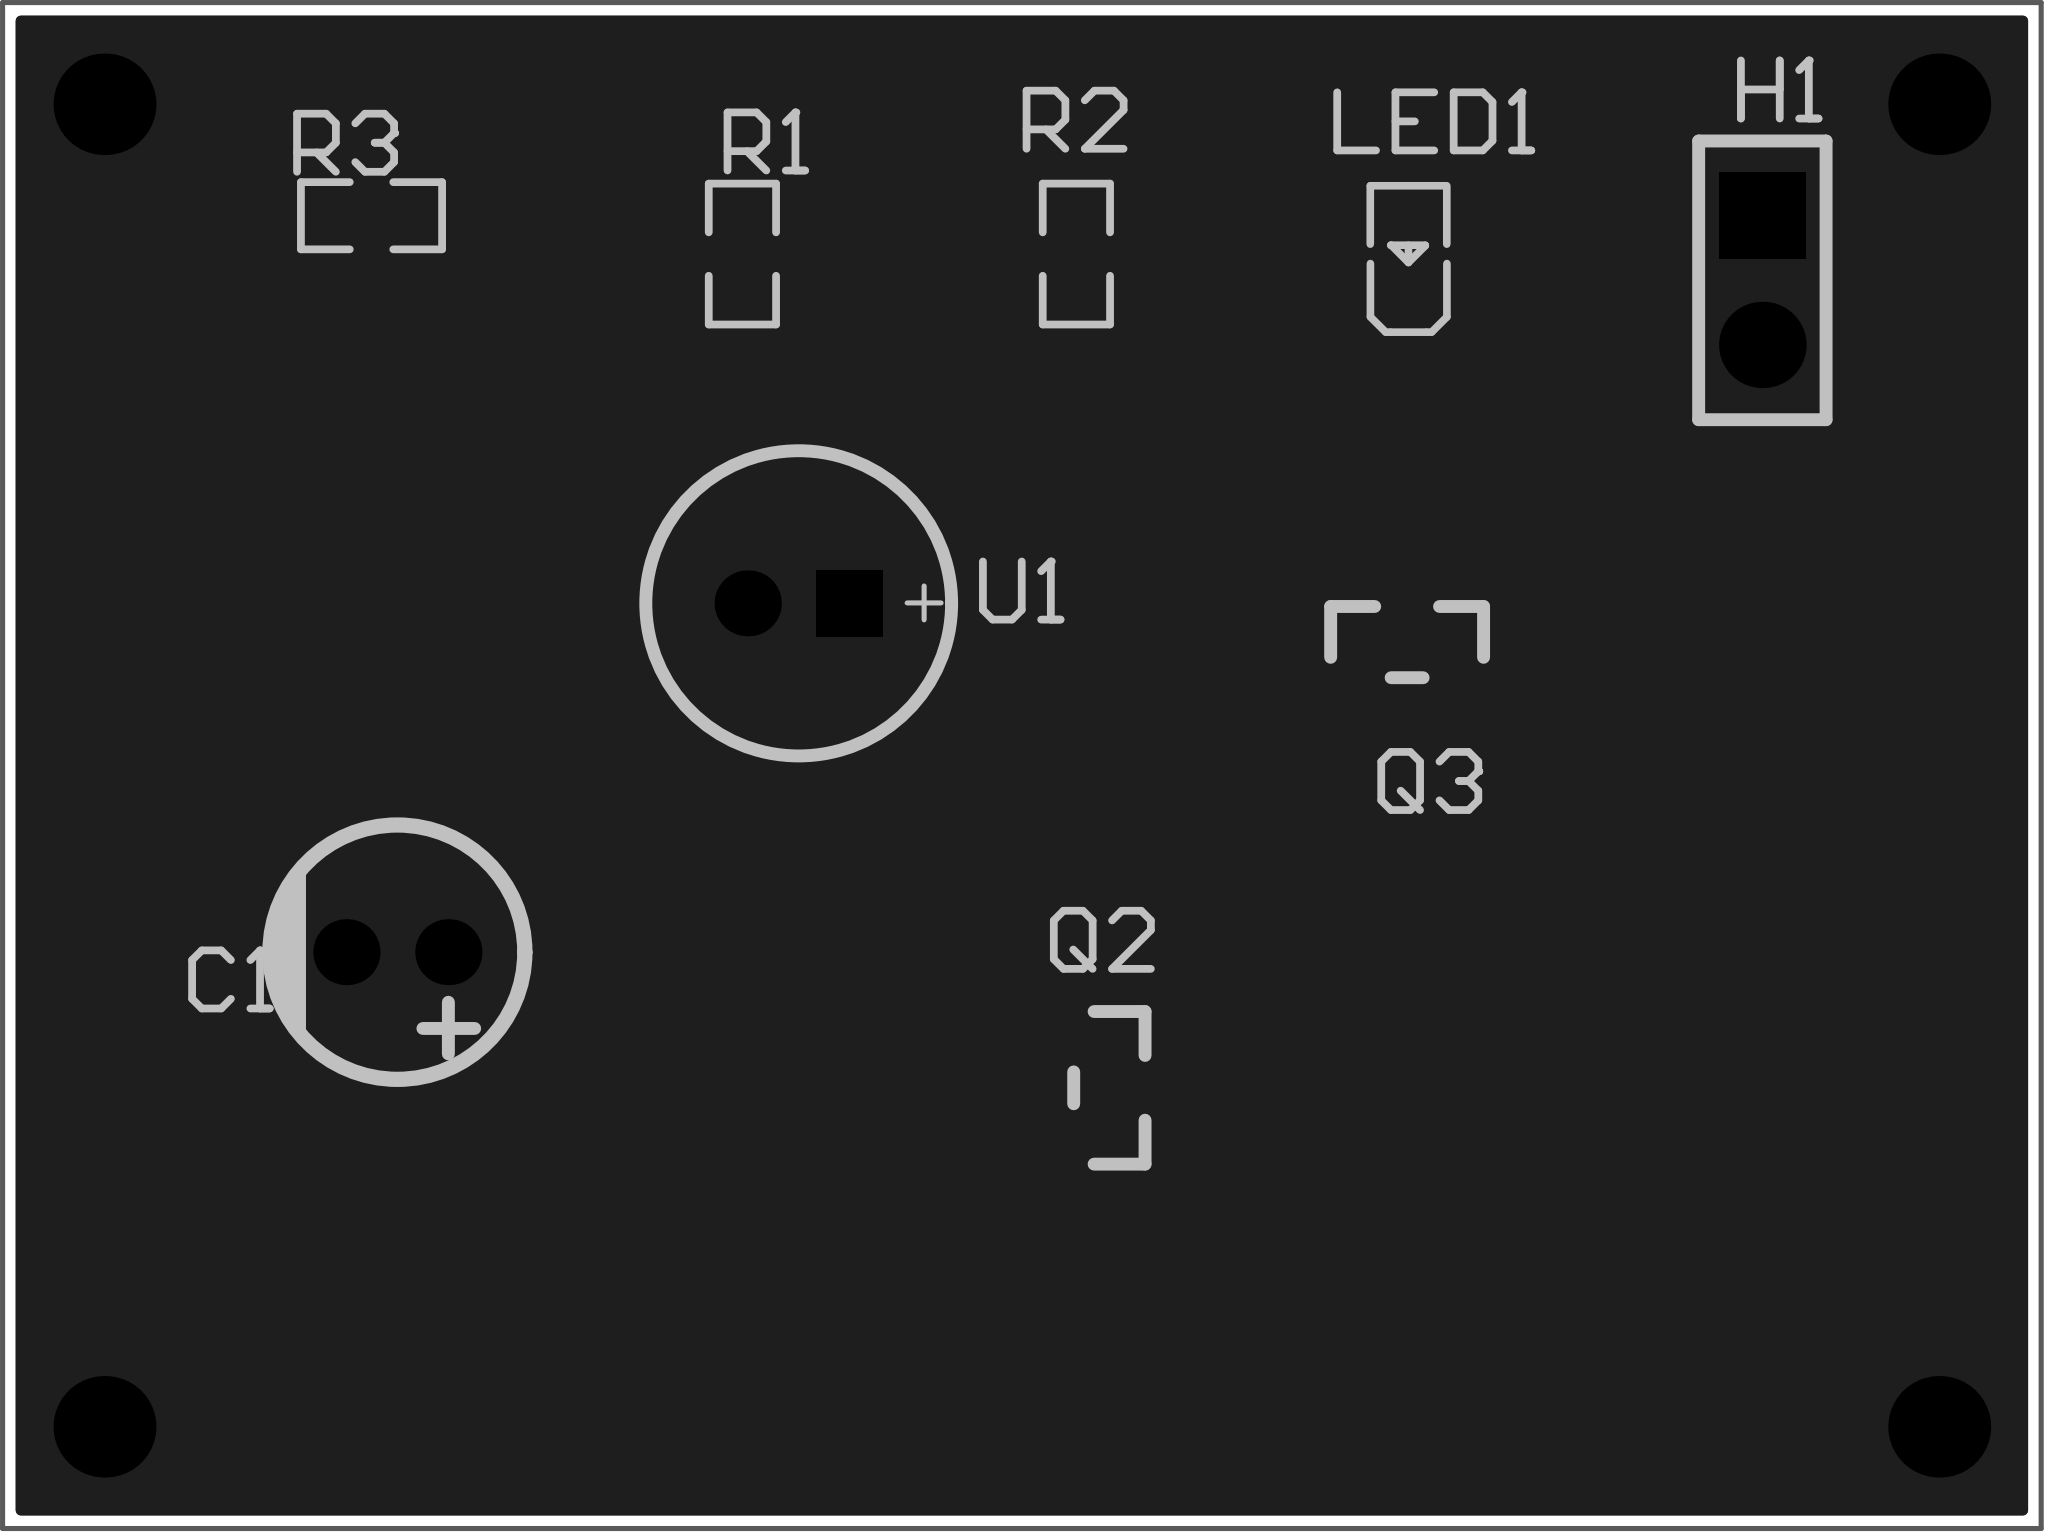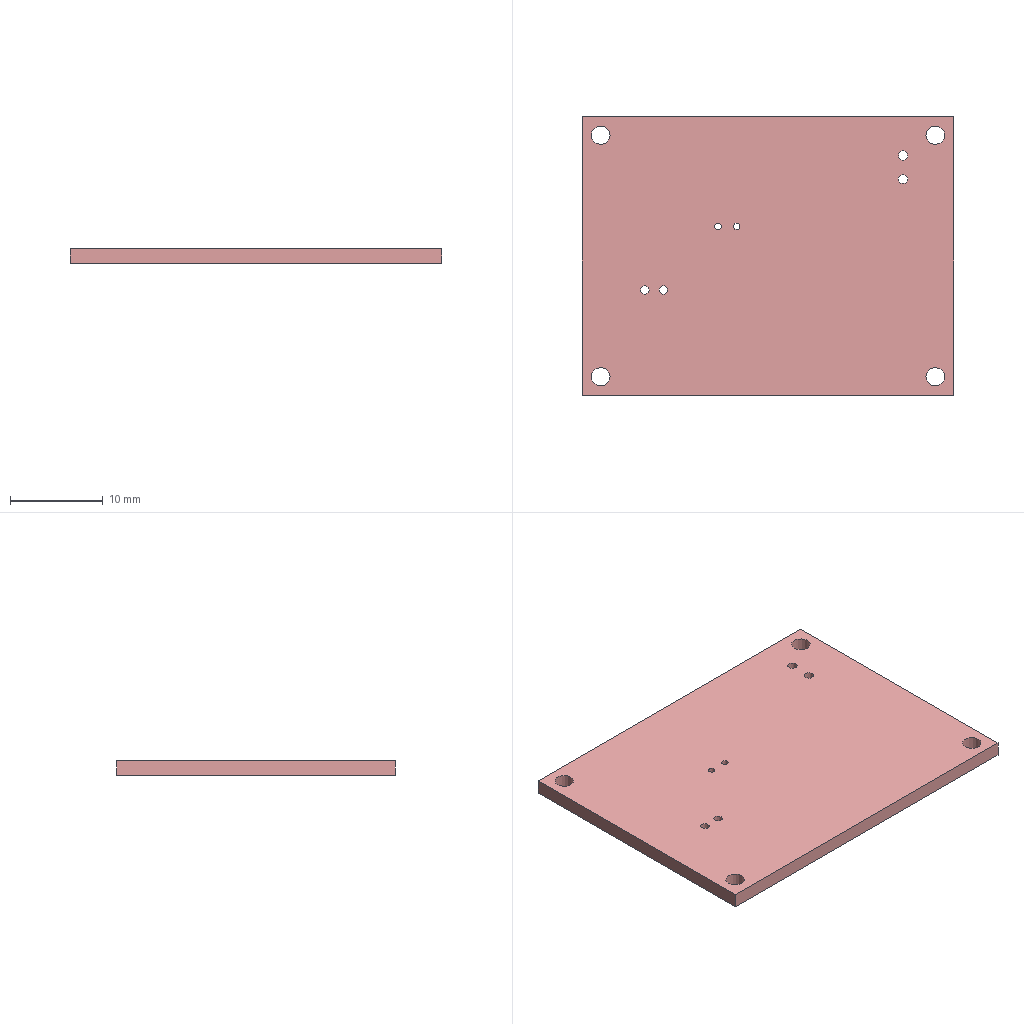Circuit board layout | Altium Designer | box 40 x 30 x 1.6 mm
Layer stack:
# Altium Designer layer stack of  (unit mm; dielectric type: 0 none, 1 core, 2 prepreg, 3 surface material)
index,name,kind,layer,copper_thickness_mm,dielectric_type,dielectric_thickness_mm,dielectric_material,dielectric_constant
0,Top Paste Mask Layer,other,,,,,,
1,Top Silkscreen Layer,other,,,,,,
2,Top Solder Mask Layer,dielectric,,,3,0.01,,3.3
3,Top Layer,copper,Top Layer,0.035,,,,
4,Dielectric1,dielectric,,,3,1.51,FR4,4.5
5,Bottom Layer,copper,Bottom Layer,0.035,,,,
6,Bottom Solder Mask Layer,dielectric,,,3,0.01,,3.3
7,Bottom Silkscreen Layer,other,,,,,,
8,Bottom Paste Mask Layer,other,,,,,,
# drill layer pairs: low layer,high layer
drill_pair,Top Layer,Bottom Layer
Part placement:
Designator,Comment,Layer,Footprint,Center-X(mm),Center-Y(mm),Rotation
C1,10uF,TopLayer,CAP-TH_BD5.0-P2.00-D0.8-FD-10UF50VC110GL,88.9,91.948,180
Q2,,TopLayer,S8050_SOT-23,102.87,89.281,180
R2,10K,TopLayer,R0603,102.222,105.673,90
R1,150K,TopLayer,R0603,95.669,105.673,90
Q3,,TopLayer,S8050_SOT-23,108.712,98.044,270
U1,电流源,TopLayer,咪头,96.774,98.806,180
LED1,,TopLayer,LED_0603,108.746,105.626,90
H1,,TopLayer,HDR-TH_2P-P2.54-V-F,115.682,105.156,270
R3,1M,TopLayer,R0603,88.392,106.426,0
Pad and via stacks:
# Altium Designer via and pad stacks of  (unit mm). Each distinct definition once, with the count of objects using it.
# via: kind,start_layer,end_layer,hole_mm,diameter_mm,mode(0 simple;1 top-mid-bottom;2 full stack),diameter_per_layer,count,example_net
# pad: kind,layer,hole_mm,hole_type(0 round;1 square;2 slot),plating,top_size,top_shape(1 round;2 rect;3 octagon;9 rounded rect),mid_size,bottom_size,mode,footprint,size_per_layer,count,example
pad,Multi-Layer,0.9,0,plated,1.3x1.3,1,1.3x1.3,1.3x1.3,0,CAP-TH_BD5.0-P2.00-D0.8-FD-10UF50VC110GL,,2,C1.2
pad,Multi-Layer,2,0,plated,2x2,1,2x2,2x2,0,,,4,1
pad,Multi-Layer,0.7,0,plated,1.3x1.3,2,1.3x1.3,1.3x1.3,0,\u00DF\u00E4\u00CD\u00B7,,1,U1.1
pad,Multi-Layer,0.7,0,plated,1.3x1.3,1,1.3x1.3,1.3x1.3,0,\u00DF\u00E4\u00CD\u00B7,,1,U1.2
pad,Multi-Layer,1,0,plated,1.7x1.7,2,1.7x1.7,1.7x1.7,0,HDR-TH_2P-P2.54-V-F,,1,H1.1
pad,Multi-Layer,1,0,plated,1.7x1.7,1,1.7x1.7,1.7x1.7,0,HDR-TH_2P-P2.54-V-F,,1,H1.2
pad,Top Layer,0,0,plated,1x0.8,2,1x0.8,1x0.8,0,S8050_SOT-23,,6,Q2.2
pad,Top Layer,0,0,plated,0.8065x0.864,2,0.8065x0.864,0.8065x0.864,0,R0603,,6,R2.2
pad,Top Layer,0,0,plated,0.8001x0.8001,2,0.8001x0.8001,0.8001x0.8001,0,LED_0603,,2,LED1.1
Copper pours:
name,layer,net,type(0 solid;1 hatched;2 none)
Top Layer-GND,Top Layer,GND,0
Bottom Layer-GND,Bottom Layer,GND,0
Design rules, without the lines most boards share:
# Altium Designer design rules of  (exported by Altium Designer, unit mm)
# columns: name | kind | enabled | priority | scope1 | scope2 | descriptor | typed fields (field=value)
creepage | 65 | enabled | 1 | All | All | Creepage Distance Constraint =(0mil) (All),(All) |